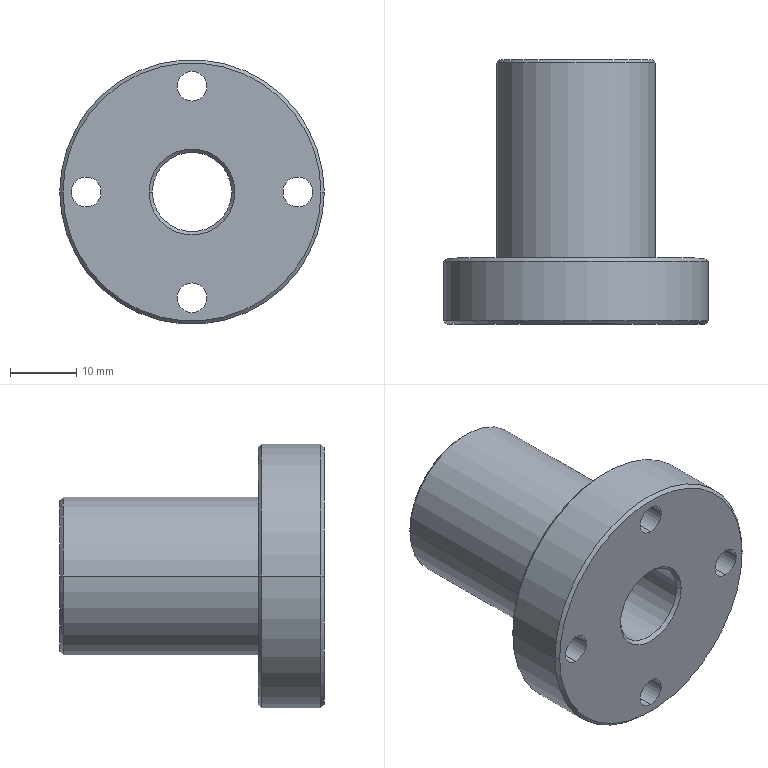Part | Creo | features DATUM PLANE 3, CURVE 2, CHAMFER 1, COORDINATE SYSTEM 1, CUT 1, PROTRUSION 1 | 1 solid | 27 faces | box 40 x 40 x 40 mm | volume 20928 mm3 | cylinder 14 | cone 10 | plane 3 | commonest cylinder face diameters 4.5 x8 12 x2 24 x2 40 x2
STEP:
#1=CARTESIAN_POINT('',(0.,0.,0.));
#2=DIRECTION('',(0.,0.,1.));
#3=DIRECTION('',(1.,0.,0.));
#4=AXIS2_PLACEMENT_3D('',#1,#2,#3);
#5=CARTESIAN_POINT('',(6.,0.5,0.));
#6=VERTEX_POINT('',#5);
#7=CARTESIAN_POINT('',(-6.,0.5,0.));
#8=VERTEX_POINT('',#7);
#9=CARTESIAN_POINT('',(0.,0.5,0.));
#10=DIRECTION('',(0.,1.,0.));
#11=DIRECTION('',(1.,0.,0.));
#12=AXIS2_PLACEMENT_3D('',#9,#10,#11);
#13=CIRCLE('',#12,6.);
#14=EDGE_CURVE('',#6,#8,#13,.T.);
#15=ORIENTED_EDGE('',*,*,#14,.T.);
#16=CARTESIAN_POINT('',(-6.,39.5,0.));
#17=VERTEX_POINT('',#16);
#18=CARTESIAN_POINT('',(-6.,39.5,-0.000000001));
#19=DIRECTION('',(0.,-1.,0.));
#20=VECTOR('',#19,39.);
#21=LINE('',#18,#20);
#22=EDGE_CURVE('',#17,#8,#21,.T.);
#23=ORIENTED_EDGE('',*,*,#22,.F.);
#24=CARTESIAN_POINT('',(6.,39.5,0.));
#25=VERTEX_POINT('',#24);
#26=CARTESIAN_POINT('',(0.,39.5,0.));
#27=DIRECTION('',(0.,1.,0.));
#28=DIRECTION('',(1.,0.,0.));
#29=AXIS2_PLACEMENT_3D('',#26,#27,#28);
#30=CIRCLE('',#29,6.);
#31=EDGE_CURVE('',#25,#17,#30,.T.);
#32=ORIENTED_EDGE('',*,*,#31,.F.);
#33=CARTESIAN_POINT('',(6.,39.5,0.000000001));
#34=DIRECTION('',(0.,-1.,0.));
#35=VECTOR('',#34,39.);
#36=LINE('',#33,#35);
#37=EDGE_CURVE('',#25,#6,#36,.T.);
#38=ORIENTED_EDGE('',*,*,#37,.T.);
#39=EDGE_LOOP('',(#15,#23,#32,#38));
#40=FACE_OUTER_BOUND('',#39,.F.);
#41=CARTESIAN_POINT('',(0.,0.,0.));
#42=DIRECTION('',(0.,1.,0.));
#43=DIRECTION('',(1.,0.,0.));
#44=AXIS2_PLACEMENT_3D('',#41,#42,#43);
#45=CYLINDRICAL_SURFACE('',#44,6.);
#46=ADVANCED_FACE('',(#40),#45,.F.);
#47=CARTESIAN_POINT('',(6.5,0.,0.));
#48=VERTEX_POINT('',#47);
#49=CARTESIAN_POINT('',(-6.5,0.,0.));
#50=VERTEX_POINT('',#49);
#51=CARTESIAN_POINT('',(0.,0.,0.));
#52=DIRECTION('',(0.,1.,0.));
#53=DIRECTION('',(1.,0.,0.));
#54=AXIS2_PLACEMENT_3D('',#51,#52,#53);
#55=CIRCLE('',#54,6.5);
#56=EDGE_CURVE('',#48,#50,#55,.T.);
#57=ORIENTED_EDGE('',*,*,#56,.T.);
#58=CARTESIAN_POINT('',(-6.5,0.000000002,0.000000002));
#59=DIRECTION('',(0.7071,0.7071,-0.000000001));
#60=VECTOR('',#59,0.7071);
#61=LINE('',#58,#60);
#62=EDGE_CURVE('',#50,#8,#61,.T.);
#63=ORIENTED_EDGE('',*,*,#62,.T.);
#64=ORIENTED_EDGE('',*,*,#14,.F.);
#65=CARTESIAN_POINT('',(6.5,0.000000002,-0.000000002));
#66=DIRECTION('',(-0.7071,0.7071,0.000000001));
#67=VECTOR('',#66,0.7071);
#68=LINE('',#65,#67);
#69=EDGE_CURVE('',#48,#6,#68,.T.);
#70=ORIENTED_EDGE('',*,*,#69,.F.);
#71=EDGE_LOOP('',(#57,#63,#64,#70));
#72=FACE_OUTER_BOUND('',#71,.F.);
#73=CARTESIAN_POINT('',(0.,0.25,0.));
#74=DIRECTION('',(0.,-1.,0.));
#75=DIRECTION('',(0.,0.,-1.));
#76=AXIS2_PLACEMENT_3D('',#73,#74,#75);
#77=CONICAL_SURFACE('',#76,6.25,45.);
#78=ADVANCED_FACE('',(#72),#77,.F.);
#79=CARTESIAN_POINT('',(-19.5,0.,0.));
#80=VERTEX_POINT('',#79);
#81=CARTESIAN_POINT('',(19.5,0.,0.));
#82=VERTEX_POINT('',#81);
#83=CARTESIAN_POINT('',(0.,0.,0.));
#84=DIRECTION('',(0.,1.,0.));
#85=DIRECTION('',(-1.,0.,0.));
#86=AXIS2_PLACEMENT_3D('',#83,#84,#85);
#87=CIRCLE('',#86,19.5);
#88=EDGE_CURVE('',#80,#82,#87,.T.);
#89=ORIENTED_EDGE('',*,*,#88,.T.);
#90=CARTESIAN_POINT('',(0.,0.,0.));
#91=DIRECTION('',(0.,1.,0.));
#92=DIRECTION('',(1.,0.,0.));
#93=AXIS2_PLACEMENT_3D('',#90,#91,#92);
#94=CIRCLE('',#93,19.5);
#95=EDGE_CURVE('',#82,#80,#94,.T.);
#96=ORIENTED_EDGE('',*,*,#95,.T.);
#97=EDGE_LOOP('',(#89,#96));
#98=FACE_OUTER_BOUND('',#97,.F.);
#99=CARTESIAN_POINT('',(0.,0.,-18.25));
#100=VERTEX_POINT('',#99);
#101=CARTESIAN_POINT('',(0.,0.,-13.75));
#102=VERTEX_POINT('',#101);
#103=CARTESIAN_POINT('',(0.,0.,-16.));
#104=DIRECTION('',(0.,-1.,0.));
#105=DIRECTION('',(0.,0.,-1.));
#106=AXIS2_PLACEMENT_3D('',#103,#104,#105);
#107=CIRCLE('',#106,2.25);
#108=EDGE_CURVE('',#100,#102,#107,.T.);
#109=ORIENTED_EDGE('',*,*,#108,.T.);
#110=CARTESIAN_POINT('',(0.,0.,-16.));
#111=DIRECTION('',(0.,-1.,0.));
#112=DIRECTION('',(0.,0.,1.));
#113=AXIS2_PLACEMENT_3D('',#110,#111,#112);
#114=CIRCLE('',#113,2.25);
#115=EDGE_CURVE('',#102,#100,#114,.T.);
#116=ORIENTED_EDGE('',*,*,#115,.T.);
#117=EDGE_LOOP('',(#109,#116));
#118=FACE_BOUND('',#117,.F.);
#119=CARTESIAN_POINT('',(0.,0.,13.75));
#120=VERTEX_POINT('',#119);
#121=CARTESIAN_POINT('',(0.,0.,18.25));
#122=VERTEX_POINT('',#121);
#123=CARTESIAN_POINT('',(0.,0.,16.));
#124=DIRECTION('',(0.,-1.,0.));
#125=DIRECTION('',(0.,0.,-1.));
#126=AXIS2_PLACEMENT_3D('',#123,#124,#125);
#127=CIRCLE('',#126,2.25);
#128=EDGE_CURVE('',#120,#122,#127,.T.);
#129=ORIENTED_EDGE('',*,*,#128,.T.);
#130=CARTESIAN_POINT('',(0.,0.,16.));
#131=DIRECTION('',(0.,-1.,0.));
#132=DIRECTION('',(0.,0.,1.));
#133=AXIS2_PLACEMENT_3D('',#130,#131,#132);
#134=CIRCLE('',#133,2.25);
#135=EDGE_CURVE('',#122,#120,#134,.T.);
#136=ORIENTED_EDGE('',*,*,#135,.T.);
#137=EDGE_LOOP('',(#129,#136));
#138=FACE_BOUND('',#137,.F.);
#139=CARTESIAN_POINT('',(-16.,0.,-2.25));
#140=VERTEX_POINT('',#139);
#141=CARTESIAN_POINT('',(-16.,0.,2.25));
#142=VERTEX_POINT('',#141);
#143=CARTESIAN_POINT('',(-16.,0.,0.));
#144=DIRECTION('',(0.,-1.,0.));
#145=DIRECTION('',(0.,0.,-1.));
#146=AXIS2_PLACEMENT_3D('',#143,#144,#145);
#147=CIRCLE('',#146,2.25);
#148=EDGE_CURVE('',#140,#142,#147,.T.);
#149=ORIENTED_EDGE('',*,*,#148,.T.);
#150=CARTESIAN_POINT('',(-16.,0.,0.));
#151=DIRECTION('',(0.,-1.,0.));
#152=DIRECTION('',(0.,0.,1.));
#153=AXIS2_PLACEMENT_3D('',#150,#151,#152);
#154=CIRCLE('',#153,2.25);
#155=EDGE_CURVE('',#142,#140,#154,.T.);
#156=ORIENTED_EDGE('',*,*,#155,.T.);
#157=EDGE_LOOP('',(#149,#156));
#158=FACE_BOUND('',#157,.F.);
#159=CARTESIAN_POINT('',(16.,0.,-2.25));
#160=VERTEX_POINT('',#159);
#161=CARTESIAN_POINT('',(16.,0.,2.25));
#162=VERTEX_POINT('',#161);
#163=CARTESIAN_POINT('',(16.,0.,0.));
#164=DIRECTION('',(0.,-1.,0.));
#165=DIRECTION('',(0.,0.,-1.));
#166=AXIS2_PLACEMENT_3D('',#163,#164,#165);
#167=CIRCLE('',#166,2.25);
#168=EDGE_CURVE('',#160,#162,#167,.T.);
#169=ORIENTED_EDGE('',*,*,#168,.T.);
#170=CARTESIAN_POINT('',(16.,0.,0.));
#171=DIRECTION('',(0.,-1.,0.));
#172=DIRECTION('',(0.,0.,1.));
#173=AXIS2_PLACEMENT_3D('',#170,#171,#172);
#174=CIRCLE('',#173,2.25);
#175=EDGE_CURVE('',#162,#160,#174,.T.);
#176=ORIENTED_EDGE('',*,*,#175,.T.);
#177=EDGE_LOOP('',(#169,#176));
#178=FACE_BOUND('',#177,.F.);
#179=ORIENTED_EDGE('',*,*,#56,.F.);
#180=CARTESIAN_POINT('',(0.,0.,0.));
#181=DIRECTION('',(0.,1.,0.));
#182=DIRECTION('',(-1.,0.,0.));
#183=AXIS2_PLACEMENT_3D('',#180,#181,#182);
#184=CIRCLE('',#183,6.5);
#185=EDGE_CURVE('',#50,#48,#184,.T.);
#186=ORIENTED_EDGE('',*,*,#185,.F.);
#187=EDGE_LOOP('',(#179,#186));
#188=FACE_BOUND('',#187,.F.);
#189=CARTESIAN_POINT('',(0.,0.,0.));
#190=DIRECTION('',(0.,1.,0.));
#191=DIRECTION('',(1.,0.,0.));
#192=AXIS2_PLACEMENT_3D('',#189,#190,#191);
#193=PLANE('',#192);
#194=ADVANCED_FACE('',(#98,#118,#138,#158,#178,#188),#193,.F.);
#195=ORIENTED_EDGE('',*,*,#168,.F.);
#196=CARTESIAN_POINT('',(16.,10.,-2.25));
#197=VERTEX_POINT('',#196);
#198=CARTESIAN_POINT('',(16.,0.,-2.25));
#199=DIRECTION('',(0.,1.,0.));
#200=VECTOR('',#199,10.);
#201=LINE('',#198,#200);
#202=EDGE_CURVE('',#160,#197,#201,.T.);
#203=ORIENTED_EDGE('',*,*,#202,.T.);
#204=CARTESIAN_POINT('',(16.,10.,2.25));
#205=VERTEX_POINT('',#204);
#206=CARTESIAN_POINT('',(16.,10.,0.));
#207=DIRECTION('',(0.,-1.,0.));
#208=DIRECTION('',(0.,0.,-1.));
#209=AXIS2_PLACEMENT_3D('',#206,#207,#208);
#210=CIRCLE('',#209,2.25);
#211=EDGE_CURVE('',#197,#205,#210,.T.);
#212=ORIENTED_EDGE('',*,*,#211,.T.);
#213=CARTESIAN_POINT('',(16.,0.,2.25));
#214=DIRECTION('',(0.,1.,0.));
#215=VECTOR('',#214,10.);
#216=LINE('',#213,#215);
#217=EDGE_CURVE('',#162,#205,#216,.T.);
#218=ORIENTED_EDGE('',*,*,#217,.F.);
#219=EDGE_LOOP('',(#195,#203,#212,#218));
#220=FACE_OUTER_BOUND('',#219,.F.);
#221=CARTESIAN_POINT('',(16.,0.,0.));
#222=DIRECTION('',(0.,-1.,0.));
#223=DIRECTION('',(0.,0.,-1.));
#224=AXIS2_PLACEMENT_3D('',#221,#222,#223);
#225=CYLINDRICAL_SURFACE('',#224,2.25);
#226=ADVANCED_FACE('',(#220),#225,.F.);
#227=ORIENTED_EDGE('',*,*,#175,.F.);
#228=ORIENTED_EDGE('',*,*,#217,.T.);
#229=CARTESIAN_POINT('',(16.,10.,0.));
#230=DIRECTION('',(0.,-1.,0.));
#231=DIRECTION('',(0.,0.,1.));
#232=AXIS2_PLACEMENT_3D('',#229,#230,#231);
#233=CIRCLE('',#232,2.25);
#234=EDGE_CURVE('',#205,#197,#233,.T.);
#235=ORIENTED_EDGE('',*,*,#234,.T.);
#236=ORIENTED_EDGE('',*,*,#202,.F.);
#237=EDGE_LOOP('',(#227,#228,#235,#236));
#238=FACE_OUTER_BOUND('',#237,.F.);
#239=CARTESIAN_POINT('',(16.,0.,0.));
#240=DIRECTION('',(0.,-1.,0.));
#241=DIRECTION('',(0.,0.,-1.));
#242=AXIS2_PLACEMENT_3D('',#239,#240,#241);
#243=CYLINDRICAL_SURFACE('',#242,2.25);
#244=ADVANCED_FACE('',(#238),#243,.F.);
#245=CARTESIAN_POINT('',(-19.5,10.,0.));
#246=VERTEX_POINT('',#245);
#247=CARTESIAN_POINT('',(19.5,10.,0.));
#248=VERTEX_POINT('',#247);
#249=CARTESIAN_POINT('',(0.,10.,0.));
#250=DIRECTION('',(0.,1.,0.));
#251=DIRECTION('',(-1.,0.,0.));
#252=AXIS2_PLACEMENT_3D('',#249,#250,#251);
#253=CIRCLE('',#252,19.5);
#254=EDGE_CURVE('',#246,#248,#253,.T.);
#255=ORIENTED_EDGE('',*,*,#254,.F.);
#256=CARTESIAN_POINT('',(0.,10.,0.));
#257=DIRECTION('',(0.,1.,0.));
#258=DIRECTION('',(1.,0.,0.));
#259=AXIS2_PLACEMENT_3D('',#256,#257,#258);
#260=CIRCLE('',#259,19.5);
#261=EDGE_CURVE('',#248,#246,#260,.T.);
#262=ORIENTED_EDGE('',*,*,#261,.F.);
#263=EDGE_LOOP('',(#255,#262));
#264=FACE_OUTER_BOUND('',#263,.F.);
#265=ORIENTED_EDGE('',*,*,#211,.F.);
#266=ORIENTED_EDGE('',*,*,#234,.F.);
#267=EDGE_LOOP('',(#265,#266));
#268=FACE_BOUND('',#267,.F.);
#269=CARTESIAN_POINT('',(0.,10.,-18.25));
#270=VERTEX_POINT('',#269);
#271=CARTESIAN_POINT('',(0.,10.,-13.75));
#272=VERTEX_POINT('',#271);
#273=CARTESIAN_POINT('',(0.,10.,-16.));
#274=DIRECTION('',(0.,-1.,0.));
#275=DIRECTION('',(0.,0.,-1.));
#276=AXIS2_PLACEMENT_3D('',#273,#274,#275);
#277=CIRCLE('',#276,2.25);
#278=EDGE_CURVE('',#270,#272,#277,.T.);
#279=ORIENTED_EDGE('',*,*,#278,.F.);
#280=CARTESIAN_POINT('',(0.,10.,-16.));
#281=DIRECTION('',(0.,-1.,0.));
#282=DIRECTION('',(0.,0.,1.));
#283=AXIS2_PLACEMENT_3D('',#280,#281,#282);
#284=CIRCLE('',#283,2.25);
#285=EDGE_CURVE('',#272,#270,#284,.T.);
#286=ORIENTED_EDGE('',*,*,#285,.F.);
#287=EDGE_LOOP('',(#279,#286));
#288=FACE_BOUND('',#287,.F.);
#289=CARTESIAN_POINT('',(0.,10.,13.75));
#290=VERTEX_POINT('',#289);
#291=CARTESIAN_POINT('',(0.,10.,18.25));
#292=VERTEX_POINT('',#291);
#293=CARTESIAN_POINT('',(0.,10.,16.));
#294=DIRECTION('',(0.,-1.,0.));
#295=DIRECTION('',(0.,0.,-1.));
#296=AXIS2_PLACEMENT_3D('',#293,#294,#295);
#297=CIRCLE('',#296,2.25);
#298=EDGE_CURVE('',#290,#292,#297,.T.);
#299=ORIENTED_EDGE('',*,*,#298,.F.);
#300=CARTESIAN_POINT('',(0.,10.,16.));
#301=DIRECTION('',(0.,-1.,0.));
#302=DIRECTION('',(0.,0.,1.));
#303=AXIS2_PLACEMENT_3D('',#300,#301,#302);
#304=CIRCLE('',#303,2.25);
#305=EDGE_CURVE('',#292,#290,#304,.T.);
#306=ORIENTED_EDGE('',*,*,#305,.F.);
#307=EDGE_LOOP('',(#299,#306));
#308=FACE_BOUND('',#307,.F.);
#309=CARTESIAN_POINT('',(-16.,10.,-2.25));
#310=VERTEX_POINT('',#309);
#311=CARTESIAN_POINT('',(-16.,10.,2.25));
#312=VERTEX_POINT('',#311);
#313=CARTESIAN_POINT('',(-16.,10.,0.));
#314=DIRECTION('',(0.,-1.,0.));
#315=DIRECTION('',(0.,0.,-1.));
#316=AXIS2_PLACEMENT_3D('',#313,#314,#315);
#317=CIRCLE('',#316,2.25);
#318=EDGE_CURVE('',#310,#312,#317,.T.);
#319=ORIENTED_EDGE('',*,*,#318,.F.);
#320=CARTESIAN_POINT('',(-16.,10.,0.));
#321=DIRECTION('',(0.,-1.,0.));
#322=DIRECTION('',(0.,0.,1.));
#323=AXIS2_PLACEMENT_3D('',#320,#321,#322);
#324=CIRCLE('',#323,2.25);
#325=EDGE_CURVE('',#312,#310,#324,.T.);
#326=ORIENTED_EDGE('',*,*,#325,.F.);
#327=EDGE_LOOP('',(#319,#326));
#328=FACE_BOUND('',#327,.F.);
#329=CARTESIAN_POINT('',(12.,10.,0.));
#330=VERTEX_POINT('',#329);
#331=CARTESIAN_POINT('',(-12.,10.,0.));
#332=VERTEX_POINT('',#331);
#333=CARTESIAN_POINT('',(0.,10.,0.));
#334=DIRECTION('',(0.,-1.,0.));
#335=DIRECTION('',(1.,0.,0.));
#336=AXIS2_PLACEMENT_3D('',#333,#334,#335);
#337=CIRCLE('',#336,12.);
#338=EDGE_CURVE('',#330,#332,#337,.T.);
#339=ORIENTED_EDGE('',*,*,#338,.F.);
#340=CARTESIAN_POINT('',(0.,10.,0.));
#341=DIRECTION('',(0.,1.,0.));
#342=DIRECTION('',(1.,0.,0.));
#343=AXIS2_PLACEMENT_3D('',#340,#341,#342);
#344=CIRCLE('',#343,12.);
#345=EDGE_CURVE('',#330,#332,#344,.T.);
#346=ORIENTED_EDGE('',*,*,#345,.T.);
#347=EDGE_LOOP('',(#339,#346));
#348=FACE_BOUND('',#347,.F.);
#349=CARTESIAN_POINT('',(0.,10.,0.));
#350=DIRECTION('',(0.,1.,0.));
#351=DIRECTION('',(1.,0.,0.));
#352=AXIS2_PLACEMENT_3D('',#349,#350,#351);
#353=PLANE('',#352);
#354=ADVANCED_FACE('',(#264,#268,#288,#308,#328,#348),#353,.T.);
#355=CARTESIAN_POINT('',(-12.,39.5,0.));
#356=VERTEX_POINT('',#355);
#357=CARTESIAN_POINT('',(12.,39.5,0.));
#358=VERTEX_POINT('',#357);
#359=CARTESIAN_POINT('',(0.,39.5,0.));
#360=DIRECTION('',(0.,1.,0.));
#361=DIRECTION('',(-1.,0.,0.));
#362=AXIS2_PLACEMENT_3D('',#359,#360,#361);
#363=CIRCLE('',#362,12.);
#364=EDGE_CURVE('',#356,#358,#363,.T.);
#365=ORIENTED_EDGE('',*,*,#364,.T.);
#366=CARTESIAN_POINT('',(12.,10.,0.));
#367=DIRECTION('',(0.,1.,0.));
#368=VECTOR('',#367,29.5);
#369=LINE('',#366,#368);
#370=EDGE_CURVE('',#330,#358,#369,.T.);
#371=ORIENTED_EDGE('',*,*,#370,.F.);
#372=ORIENTED_EDGE('',*,*,#338,.T.);
#373=CARTESIAN_POINT('',(-12.,10.,0.));
#374=DIRECTION('',(0.,1.,0.));
#375=VECTOR('',#374,29.5);
#376=LINE('',#373,#375);
#377=EDGE_CURVE('',#332,#356,#376,.T.);
#378=ORIENTED_EDGE('',*,*,#377,.T.);
#379=EDGE_LOOP('',(#365,#371,#372,#378));
#380=FACE_OUTER_BOUND('',#379,.F.);
#381=CARTESIAN_POINT('',(0.,0.,0.));
#382=DIRECTION('',(0.,1.,0.));
#383=DIRECTION('',(1.,0.,0.));
#384=AXIS2_PLACEMENT_3D('',#381,#382,#383);
#385=CYLINDRICAL_SURFACE('',#384,12.);
#386=ADVANCED_FACE('',(#380),#385,.T.);
#387=CARTESIAN_POINT('',(-11.5,40.,0.));
#388=VERTEX_POINT('',#387);
#389=CARTESIAN_POINT('',(11.5,40.,0.));
#390=VERTEX_POINT('',#389);
#391=CARTESIAN_POINT('',(0.,40.,0.));
#392=DIRECTION('',(0.,1.,0.));
#393=DIRECTION('',(-1.,0.,0.));
#394=AXIS2_PLACEMENT_3D('',#391,#392,#393);
#395=CIRCLE('',#394,11.5);
#396=EDGE_CURVE('',#388,#390,#395,.T.);
#397=ORIENTED_EDGE('',*,*,#396,.T.);
#398=CARTESIAN_POINT('',(11.5,40.,-0.000000004));
#399=DIRECTION('',(0.7071,-0.7071,0.000000001));
#400=VECTOR('',#399,0.7071);
#401=LINE('',#398,#400);
#402=EDGE_CURVE('',#390,#358,#401,.T.);
#403=ORIENTED_EDGE('',*,*,#402,.T.);
#404=ORIENTED_EDGE('',*,*,#364,.F.);
#405=CARTESIAN_POINT('',(-11.5,40.,0.000000004));
#406=DIRECTION('',(-0.7071,-0.7071,-0.000000001));
#407=VECTOR('',#406,0.7071);
#408=LINE('',#405,#407);
#409=EDGE_CURVE('',#388,#356,#408,.T.);
#410=ORIENTED_EDGE('',*,*,#409,.F.);
#411=EDGE_LOOP('',(#397,#403,#404,#410));
#412=FACE_OUTER_BOUND('',#411,.F.);
#413=CARTESIAN_POINT('',(0.,39.75,0.));
#414=DIRECTION('',(0.,-1.,0.));
#415=DIRECTION('',(0.,0.,-1.));
#416=AXIS2_PLACEMENT_3D('',#413,#414,#415);
#417=CONICAL_SURFACE('',#416,11.75,45.);
#418=ADVANCED_FACE('',(#412),#417,.T.);
#419=ORIENTED_EDGE('',*,*,#396,.F.);
#420=CARTESIAN_POINT('',(0.,40.,0.));
#421=DIRECTION('',(0.,1.,0.));
#422=DIRECTION('',(1.,0.,0.));
#423=AXIS2_PLACEMENT_3D('',#420,#421,#422);
#424=CIRCLE('',#423,11.5);
#425=EDGE_CURVE('',#390,#388,#424,.T.);
#426=ORIENTED_EDGE('',*,*,#425,.F.);
#427=EDGE_LOOP('',(#419,#426));
#428=FACE_OUTER_BOUND('',#427,.F.);
#429=CARTESIAN_POINT('',(6.5,40.,0.));
#430=VERTEX_POINT('',#429);
#431=CARTESIAN_POINT('',(-6.5,40.,0.));
#432=VERTEX_POINT('',#431);
#433=CARTESIAN_POINT('',(0.,40.,0.));
#434=DIRECTION('',(0.,1.,0.));
#435=DIRECTION('',(1.,0.,0.));
#436=AXIS2_PLACEMENT_3D('',#433,#434,#435);
#437=CIRCLE('',#436,6.5);
#438=EDGE_CURVE('',#430,#432,#437,.T.);
#439=ORIENTED_EDGE('',*,*,#438,.T.);
#440=CARTESIAN_POINT('',(0.,40.,0.));
#441=DIRECTION('',(0.,1.,0.));
#442=DIRECTION('',(-1.,0.,0.));
#443=AXIS2_PLACEMENT_3D('',#440,#441,#442);
#444=CIRCLE('',#443,6.5);
#445=EDGE_CURVE('',#432,#430,#444,.T.);
#446=ORIENTED_EDGE('',*,*,#445,.T.);
#447=EDGE_LOOP('',(#439,#446));
#448=FACE_BOUND('',#447,.F.);
#449=CARTESIAN_POINT('',(0.,40.,0.));
#450=DIRECTION('',(0.,1.,0.));
#451=DIRECTION('',(1.,0.,0.));
#452=AXIS2_PLACEMENT_3D('',#449,#450,#451);
#453=PLANE('',#452);
#454=ADVANCED_FACE('',(#428,#448),#453,.T.);
#455=ORIENTED_EDGE('',*,*,#425,.T.);
#456=ORIENTED_EDGE('',*,*,#409,.T.);
#457=CARTESIAN_POINT('',(0.,39.5,0.));
#458=DIRECTION('',(0.,1.,0.));
#459=DIRECTION('',(1.,0.,0.));
#460=AXIS2_PLACEMENT_3D('',#457,#458,#459);
#461=CIRCLE('',#460,12.);
#462=EDGE_CURVE('',#358,#356,#461,.T.);
#463=ORIENTED_EDGE('',*,*,#462,.F.);
#464=ORIENTED_EDGE('',*,*,#402,.F.);
#465=EDGE_LOOP('',(#455,#456,#463,#464));
#466=FACE_OUTER_BOUND('',#465,.F.);
#467=CARTESIAN_POINT('',(0.,39.75,0.));
#468=DIRECTION('',(0.,-1.,0.));
#469=DIRECTION('',(0.,0.,-1.));
#470=AXIS2_PLACEMENT_3D('',#467,#468,#469);
#471=CONICAL_SURFACE('',#470,11.75,45.);
#472=ADVANCED_FACE('',(#466),#471,.T.);
#473=ORIENTED_EDGE('',*,*,#462,.T.);
#474=ORIENTED_EDGE('',*,*,#377,.F.);
#475=ORIENTED_EDGE('',*,*,#345,.F.);
#476=ORIENTED_EDGE('',*,*,#370,.T.);
#477=EDGE_LOOP('',(#473,#474,#475,#476));
#478=FACE_OUTER_BOUND('',#477,.F.);
#479=CARTESIAN_POINT('',(0.,0.,0.));
#480=DIRECTION('',(0.,1.,0.));
#481=DIRECTION('',(1.,0.,0.));
#482=AXIS2_PLACEMENT_3D('',#479,#480,#481);
#483=CYLINDRICAL_SURFACE('',#482,12.);
#484=ADVANCED_FACE('',(#478),#483,.T.);
#485=ORIENTED_EDGE('',*,*,#31,.T.);
#486=CARTESIAN_POINT('',(-6.,39.5,-0.000000001));
#487=DIRECTION('',(-0.7071,0.7071,-0.000000001));
#488=VECTOR('',#487,0.7071);
#489=LINE('',#486,#488);
#490=EDGE_CURVE('',#17,#432,#489,.T.);
#491=ORIENTED_EDGE('',*,*,#490,.T.);
#492=ORIENTED_EDGE('',*,*,#438,.F.);
#493=CARTESIAN_POINT('',(6.,39.5,0.000000001));
#494=DIRECTION('',(0.7071,0.7071,0.000000001));
#495=VECTOR('',#494,0.7071);
#496=LINE('',#493,#495);
#497=EDGE_CURVE('',#25,#430,#496,.T.);
#498=ORIENTED_EDGE('',*,*,#497,.F.);
#499=EDGE_LOOP('',(#485,#491,#492,#498));
#500=FACE_OUTER_BOUND('',#499,.F.);
#501=CARTESIAN_POINT('',(0.,39.75,0.));
#502=DIRECTION('',(0.,1.,0.));
#503=DIRECTION('',(0.,0.,-1.));
#504=AXIS2_PLACEMENT_3D('',#501,#502,#503);
#505=CONICAL_SURFACE('',#504,6.25,45.);
#506=ADVANCED_FACE('',(#500),#505,.F.);
#507=CARTESIAN_POINT('',(0.,39.5,0.));
#508=DIRECTION('',(0.,1.,0.));
#509=DIRECTION('',(-1.,0.,0.));
#510=AXIS2_PLACEMENT_3D('',#507,#508,#509);
#511=CIRCLE('',#510,6.);
#512=EDGE_CURVE('',#17,#25,#511,.T.);
#513=ORIENTED_EDGE('',*,*,#512,.T.);
#514=ORIENTED_EDGE('',*,*,#497,.T.);
#515=ORIENTED_EDGE('',*,*,#445,.F.);
#516=ORIENTED_EDGE('',*,*,#490,.F.);
#517=EDGE_LOOP('',(#513,#514,#515,#516));
#518=FACE_OUTER_BOUND('',#517,.F.);
#519=CARTESIAN_POINT('',(0.,39.75,0.));
#520=DIRECTION('',(0.,1.,0.));
#521=DIRECTION('',(0.,0.,-1.));
#522=AXIS2_PLACEMENT_3D('',#519,#520,#521);
#523=CONICAL_SURFACE('',#522,6.25,45.);
#524=ADVANCED_FACE('',(#518),#523,.F.);
#525=CARTESIAN_POINT('',(0.,0.5,0.));
#526=DIRECTION('',(0.,1.,0.));
#527=DIRECTION('',(-1.,0.,0.));
#528=AXIS2_PLACEMENT_3D('',#525,#526,#527);
#529=CIRCLE('',#528,6.);
#530=EDGE_CURVE('',#8,#6,#529,.T.);
#531=ORIENTED_EDGE('',*,*,#530,.T.);
#532=ORIENTED_EDGE('',*,*,#37,.F.);
#533=ORIENTED_EDGE('',*,*,#512,.F.);
#534=ORIENTED_EDGE('',*,*,#22,.T.);
#535=EDGE_LOOP('',(#531,#532,#533,#534));
#536=FACE_OUTER_BOUND('',#535,.F.);
#537=CARTESIAN_POINT('',(0.,0.,0.));
#538=DIRECTION('',(0.,1.,0.));
#539=DIRECTION('',(1.,0.,0.));
#540=AXIS2_PLACEMENT_3D('',#537,#538,#539);
#541=CYLINDRICAL_SURFACE('',#540,6.);
#542=ADVANCED_FACE('',(#536),#541,.F.);
#543=ORIENTED_EDGE('',*,*,#185,.T.);
#544=ORIENTED_EDGE('',*,*,#69,.T.);
#545=ORIENTED_EDGE('',*,*,#530,.F.);
#546=ORIENTED_EDGE('',*,*,#62,.F.);
#547=EDGE_LOOP('',(#543,#544,#545,#546));
#548=FACE_OUTER_BOUND('',#547,.F.);
#549=CARTESIAN_POINT('',(0.,0.25,0.));
#550=DIRECTION('',(0.,-1.,0.));
#551=DIRECTION('',(0.,0.,-1.));
#552=AXIS2_PLACEMENT_3D('',#549,#550,#551);
#553=CONICAL_SURFACE('',#552,6.25,45.);
#554=ADVANCED_FACE('',(#548),#553,.F.);
#555=ORIENTED_EDGE('',*,*,#108,.F.);
#556=CARTESIAN_POINT('',(0.,0.,-18.25));
#557=DIRECTION('',(0.,1.,0.));
#558=VECTOR('',#557,10.);
#559=LINE('',#556,#558);
#560=EDGE_CURVE('',#100,#270,#559,.T.);
#561=ORIENTED_EDGE('',*,*,#560,.T.);
#562=ORIENTED_EDGE('',*,*,#278,.T.);
#563=CARTESIAN_POINT('',(0.,0.,-13.75));
#564=DIRECTION('',(0.,1.,0.));
#565=VECTOR('',#564,10.);
#566=LINE('',#563,#565);
#567=EDGE_CURVE('',#102,#272,#566,.T.);
#568=ORIENTED_EDGE('',*,*,#567,.F.);
#569=EDGE_LOOP('',(#555,#561,#562,#568));
#570=FACE_OUTER_BOUND('',#569,.F.);
#571=CARTESIAN_POINT('',(0.,0.,-16.));
#572=DIRECTION('',(0.,-1.,0.));
#573=DIRECTION('',(0.,0.,-1.));
#574=AXIS2_PLACEMENT_3D('',#571,#572,#573);
#575=CYLINDRICAL_SURFACE('',#574,2.25);
#576=ADVANCED_FACE('',(#570),#575,.F.);
#577=ORIENTED_EDGE('',*,*,#115,.F.);
#578=ORIENTED_EDGE('',*,*,#567,.T.);
#579=ORIENTED_EDGE('',*,*,#285,.T.);
#580=ORIENTED_EDGE('',*,*,#560,.F.);
#581=EDGE_LOOP('',(#577,#578,#579,#580));
#582=FACE_OUTER_BOUND('',#581,.F.);
#583=CARTESIAN_POINT('',(0.,0.,-16.));
#584=DIRECTION('',(0.,-1.,0.));
#585=DIRECTION('',(0.,0.,-1.));
#586=AXIS2_PLACEMENT_3D('',#583,#584,#585);
#587=CYLINDRICAL_SURFACE('',#586,2.25);
#588=ADVANCED_FACE('',(#582),#587,.F.);
#589=ORIENTED_EDGE('',*,*,#128,.F.);
#590=CARTESIAN_POINT('',(0.,0.,13.75));
#591=DIRECTION('',(0.,1.,0.));
#592=VECTOR('',#591,10.);
#593=LINE('',#590,#592);
#594=EDGE_CURVE('',#120,#290,#593,.T.);
#595=ORIENTED_EDGE('',*,*,#594,.T.);
#596=ORIENTED_EDGE('',*,*,#298,.T.);
#597=CARTESIAN_POINT('',(0.,0.,18.25));
#598=DIRECTION('',(0.,1.,0.));
#599=VECTOR('',#598,10.);
#600=LINE('',#597,#599);
#601=EDGE_CURVE('',#122,#292,#600,.T.);
#602=ORIENTED_EDGE('',*,*,#601,.F.);
#603=EDGE_LOOP('',(#589,#595,#596,#602));
#604=FACE_OUTER_BOUND('',#603,.F.);
#605=CARTESIAN_POINT('',(0.,0.,16.));
#606=DIRECTION('',(0.,-1.,0.));
#607=DIRECTION('',(0.,0.,-1.));
#608=AXIS2_PLACEMENT_3D('',#605,#606,#607);
#609=CYLINDRICAL_SURFACE('',#608,2.25);
#610=ADVANCED_FACE('',(#604),#609,.F.);
#611=ORIENTED_EDGE('',*,*,#135,.F.);
#612=ORIENTED_EDGE('',*,*,#601,.T.);
#613=ORIENTED_EDGE('',*,*,#305,.T.);
#614=ORIENTED_EDGE('',*,*,#594,.F.);
#615=EDGE_LOOP('',(#611,#612,#613,#614));
#616=FACE_OUTER_BOUND('',#615,.F.);
#617=CARTESIAN_POINT('',(0.,0.,16.));
#618=DIRECTION('',(0.,-1.,0.));
#619=DIRECTION('',(0.,0.,-1.));
#620=AXIS2_PLACEMENT_3D('',#617,#618,#619);
#621=CYLINDRICAL_SURFACE('',#620,2.25);
#622=ADVANCED_FACE('',(#616),#621,.F.);
#623=ORIENTED_EDGE('',*,*,#148,.F.);
#624=CARTESIAN_POINT('',(-16.,0.,-2.25));
#625=DIRECTION('',(0.,1.,0.));
#626=VECTOR('',#625,10.);
#627=LINE('',#624,#626);
#628=EDGE_CURVE('',#140,#310,#627,.T.);
#629=ORIENTED_EDGE('',*,*,#628,.T.);
#630=ORIENTED_EDGE('',*,*,#318,.T.);
#631=CARTESIAN_POINT('',(-16.,0.,2.25));
#632=DIRECTION('',(0.,1.,0.));
#633=VECTOR('',#632,10.);
#634=LINE('',#631,#633);
#635=EDGE_CURVE('',#142,#312,#634,.T.);
#636=ORIENTED_EDGE('',*,*,#635,.F.);
#637=EDGE_LOOP('',(#623,#629,#630,#636));
#638=FACE_OUTER_BOUND('',#637,.F.);
#639=CARTESIAN_POINT('',(-16.,0.,0.));
#640=DIRECTION('',(0.,-1.,0.));
#641=DIRECTION('',(0.,0.,-1.));
#642=AXIS2_PLACEMENT_3D('',#639,#640,#641);
#643=CYLINDRICAL_SURFACE('',#642,2.25);
#644=ADVANCED_FACE('',(#638),#643,.F.);
#645=ORIENTED_EDGE('',*,*,#155,.F.);
#646=ORIENTED_EDGE('',*,*,#635,.T.);
#647=ORIENTED_EDGE('',*,*,#325,.T.);
#648=ORIENTED_EDGE('',*,*,#628,.F.);
#649=EDGE_LOOP('',(#645,#646,#647,#648));
#650=FACE_OUTER_BOUND('',#649,.F.);
#651=CARTESIAN_POINT('',(-16.,0.,0.));
#652=DIRECTION('',(0.,-1.,0.));
#653=DIRECTION('',(0.,0.,-1.));
#654=AXIS2_PLACEMENT_3D('',#651,#652,#653);
#655=CYLINDRICAL_SURFACE('',#654,2.25);
#656=ADVANCED_FACE('',(#650),#655,.F.);
#657=ORIENTED_EDGE('',*,*,#254,.T.);
#658=CARTESIAN_POINT('',(20.,9.5,0.));
#659=VERTEX_POINT('',#658);
#660=CARTESIAN_POINT('',(19.5,10.,-0.000000004));
#661=DIRECTION('',(0.7071,-0.7071,0.000000001));
#662=VECTOR('',#661,0.7071);
#663=LINE('',#660,#662);
#664=EDGE_CURVE('',#248,#659,#663,.T.);
#665=ORIENTED_EDGE('',*,*,#664,.T.);
#666=CARTESIAN_POINT('',(-20.,9.5,0.));
#667=VERTEX_POINT('',#666);
#668=CARTESIAN_POINT('',(0.,9.5,0.));
#669=DIRECTION('',(0.,1.,0.));
#670=DIRECTION('',(-1.,0.,0.));
#671=AXIS2_PLACEMENT_3D('',#668,#669,#670);
#672=CIRCLE('',#671,20.);
#673=EDGE_CURVE('',#667,#659,#672,.T.);
#674=ORIENTED_EDGE('',*,*,#673,.F.);
#675=CARTESIAN_POINT('',(-19.5,10.,0.000000004));
#676=DIRECTION('',(-0.7071,-0.7071,-0.000000001));
#677=VECTOR('',#676,0.7071);
#678=LINE('',#675,#677);
#679=EDGE_CURVE('',#246,#667,#678,.T.);
#680=ORIENTED_EDGE('',*,*,#679,.F.);
#681=EDGE_LOOP('',(#657,#665,#674,#680));
#682=FACE_OUTER_BOUND('',#681,.F.);
#683=CARTESIAN_POINT('',(0.,9.75,0.));
#684=DIRECTION('',(0.,-1.,0.));
#685=DIRECTION('',(0.,0.,-1.));
#686=AXIS2_PLACEMENT_3D('',#683,#684,#685);
#687=CONICAL_SURFACE('',#686,19.75,45.);
#688=ADVANCED_FACE('',(#682),#687,.T.);
#689=ORIENTED_EDGE('',*,*,#261,.T.);
#690=ORIENTED_EDGE('',*,*,#679,.T.);
#691=CARTESIAN_POINT('',(0.,9.5,0.));
#692=DIRECTION('',(0.,1.,0.));
#693=DIRECTION('',(1.,0.,0.));
#694=AXIS2_PLACEMENT_3D('',#691,#692,#693);
#695=CIRCLE('',#694,20.);
#696=EDGE_CURVE('',#659,#667,#695,.T.);
#697=ORIENTED_EDGE('',*,*,#696,.F.);
#698=ORIENTED_EDGE('',*,*,#664,.F.);
#699=EDGE_LOOP('',(#689,#690,#697,#698));
#700=FACE_OUTER_BOUND('',#699,.F.);
#701=CARTESIAN_POINT('',(0.,9.75,0.));
#702=DIRECTION('',(0.,-1.,0.));
#703=DIRECTION('',(0.,0.,-1.));
#704=AXIS2_PLACEMENT_3D('',#701,#702,#703);
#705=CONICAL_SURFACE('',#704,19.75,45.);
#706=ADVANCED_FACE('',(#700),#705,.T.);
#707=CARTESIAN_POINT('',(20.,0.5,0.));
#708=VERTEX_POINT('',#707);
#709=CARTESIAN_POINT('',(-20.,0.5,0.));
#710=VERTEX_POINT('',#709);
#711=CARTESIAN_POINT('',(0.,0.5,0.));
#712=DIRECTION('',(0.,1.,0.));
#713=DIRECTION('',(1.,0.,0.));
#714=AXIS2_PLACEMENT_3D('',#711,#712,#713);
#715=CIRCLE('',#714,20.);
#716=EDGE_CURVE('',#708,#710,#715,.T.);
#717=ORIENTED_EDGE('',*,*,#716,.F.);
#718=CARTESIAN_POINT('',(20.,0.5,0.000000001));
#719=DIRECTION('',(0.,1.,0.));
#720=VECTOR('',#719,9.);
#721=LINE('',#718,#720);
#722=EDGE_CURVE('',#708,#659,#721,.T.);
#723=ORIENTED_EDGE('',*,*,#722,.T.);
#724=ORIENTED_EDGE('',*,*,#696,.T.);
#725=CARTESIAN_POINT('',(-20.,0.5,-0.000000001));
#726=DIRECTION('',(0.,1.,0.));
#727=VECTOR('',#726,9.);
#728=LINE('',#725,#727);
#729=EDGE_CURVE('',#710,#667,#728,.T.);
#730=ORIENTED_EDGE('',*,*,#729,.F.);
#731=EDGE_LOOP('',(#717,#723,#724,#730));
#732=FACE_OUTER_BOUND('',#731,.F.);
#733=CARTESIAN_POINT('',(0.,0.,0.));
#734=DIRECTION('',(0.,1.,0.));
#735=DIRECTION('',(1.,0.,0.));
#736=AXIS2_PLACEMENT_3D('',#733,#734,#735);
#737=CYLINDRICAL_SURFACE('',#736,20.);
#738=ADVANCED_FACE('',(#732),#737,.T.);
#739=ORIENTED_EDGE('',*,*,#716,.T.);
#740=CARTESIAN_POINT('',(-20.,0.5,-0.000000001));
#741=DIRECTION('',(0.7071,-0.7071,0.));
#742=VECTOR('',#741,0.7071);
#743=LINE('',#740,#742);
#744=EDGE_CURVE('',#710,#80,#743,.T.);
#745=ORIENTED_EDGE('',*,*,#744,.T.);
#746=ORIENTED_EDGE('',*,*,#95,.F.);
#747=CARTESIAN_POINT('',(20.,0.5,0.000000001));
#748=DIRECTION('',(-0.7071,-0.7071,0.));
#749=VECTOR('',#748,0.7071);
#750=LINE('',#747,#749);
#751=EDGE_CURVE('',#708,#82,#750,.T.);
#752=ORIENTED_EDGE('',*,*,#751,.F.);
#753=EDGE_LOOP('',(#739,#745,#746,#752));
#754=FACE_OUTER_BOUND('',#753,.F.);
#755=CARTESIAN_POINT('',(0.,0.25,0.));
#756=DIRECTION('',(0.,1.,0.));
#757=DIRECTION('',(0.,0.,-1.));
#758=AXIS2_PLACEMENT_3D('',#755,#756,#757);
#759=CONICAL_SURFACE('',#758,19.75,45.);
#760=ADVANCED_FACE('',(#754),#759,.T.);
#761=CARTESIAN_POINT('',(0.,0.5,0.));
#762=DIRECTION('',(0.,1.,0.));
#763=DIRECTION('',(-1.,0.,0.));
#764=AXIS2_PLACEMENT_3D('',#761,#762,#763);
#765=CIRCLE('',#764,20.);
#766=EDGE_CURVE('',#710,#708,#765,.T.);
#767=ORIENTED_EDGE('',*,*,#766,.T.);
#768=ORIENTED_EDGE('',*,*,#751,.T.);
#769=ORIENTED_EDGE('',*,*,#88,.F.);
#770=ORIENTED_EDGE('',*,*,#744,.F.);
#771=EDGE_LOOP('',(#767,#768,#769,#770));
#772=FACE_OUTER_BOUND('',#771,.F.);
#773=CARTESIAN_POINT('',(0.,0.25,0.));
#774=DIRECTION('',(0.,1.,0.));
#775=DIRECTION('',(0.,0.,-1.));
#776=AXIS2_PLACEMENT_3D('',#773,#774,#775);
#777=CONICAL_SURFACE('',#776,19.75,45.);
#778=ADVANCED_FACE('',(#772),#777,.T.);
#779=ORIENTED_EDGE('',*,*,#766,.F.);
#780=ORIENTED_EDGE('',*,*,#729,.T.);
#781=ORIENTED_EDGE('',*,*,#673,.T.);
#782=ORIENTED_EDGE('',*,*,#722,.F.);
#783=EDGE_LOOP('',(#779,#780,#781,#782));
#784=FACE_OUTER_BOUND('',#783,.F.);
#785=CARTESIAN_POINT('',(0.,0.,0.));
#786=DIRECTION('',(0.,1.,0.));
#787=DIRECTION('',(1.,0.,0.));
#788=AXIS2_PLACEMENT_3D('',#785,#786,#787);
#789=CYLINDRICAL_SURFACE('',#788,20.);
#790=ADVANCED_FACE('',(#784),#789,.T.);
#791=CLOSED_SHELL('',(#46,#78,#194,#226,#244,#354,#386,#418,#454,#472,#484,#506,#524,#542,#554,#576,#588,#610,#622,#644,#656,#688,#706,#738,#760,#778,#790));
#792=MANIFOLD_SOLID_BREP('',#791);
#793=(LENGTH_UNIT()NAMED_UNIT(*)SI_UNIT(.MILLI.,.METRE.));
#794=UNCERTAINTY_MEASURE_WITH_UNIT(LENGTH_MEASURE(0.00693),#793,'','');
#795=(NAMED_UNIT(*)PLANE_ANGLE_UNIT()SI_UNIT($,.RADIAN.));
#796=PLANE_ANGLE_MEASURE_WITH_UNIT(PLANE_ANGLE_MEASURE(0.01745),#795);
#797=(CONVERSION_BASED_UNIT('DEGREE',#796)NAMED_UNIT(*)PLANE_ANGLE_UNIT());
#798=(NAMED_UNIT(*)SI_UNIT($,.STERADIAN.)SOLID_ANGLE_UNIT());
#799=(GEOMETRIC_REPRESENTATION_CONTEXT(3)GLOBAL_UNCERTAINTY_ASSIGNED_CONTEXT((#794))GLOBAL_UNIT_ASSIGNED_CONTEXT((#793,#797,#798))REPRESENTATION_CONTEXT('',''));
#800=ADVANCED_BREP_SHAPE_REPRESENTATION('',(#4,#792),#799);